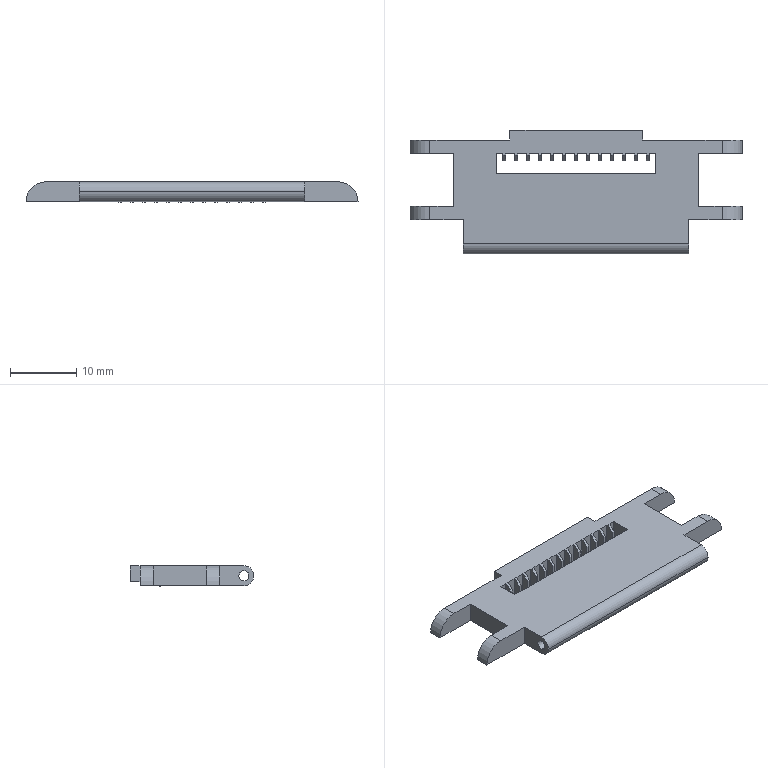Part | SolidWorks | features ICE 11, Chamfer 2, Fillet 2, LPattern 2, Extrusion 1, MirrorPattern 1, MoveFace 1 | 1 solid | 120 faces | box 50 x 18.64 x 3.07 mm | volume 1775 mm3 | plane 112 | cylinder 8 | commonest cylinder face diameters 6 x4 1.5 x2 3 x2